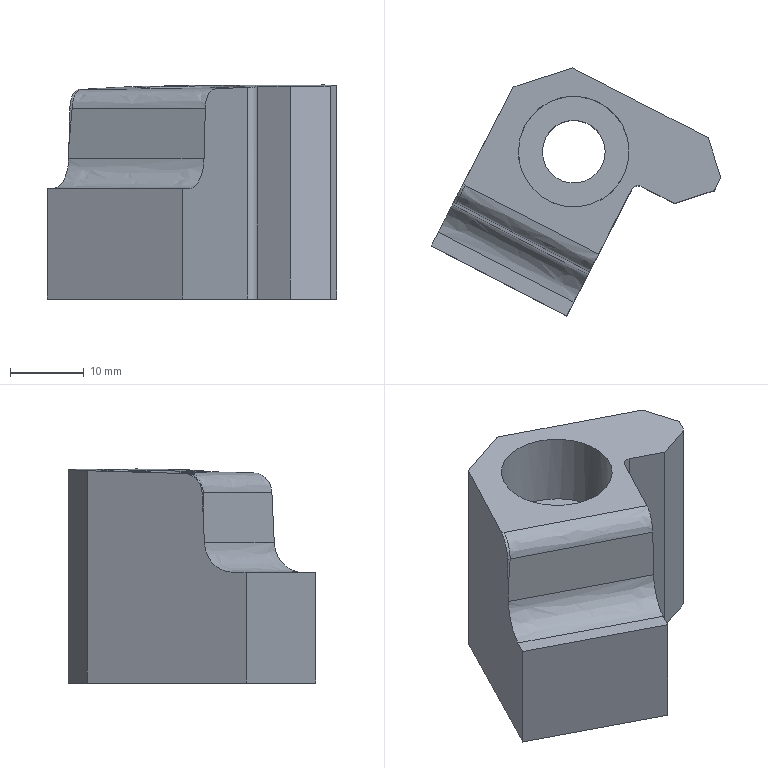Part | STEP file | gslz 2016.10.28-13_id1634_x_t | 1 solid | 21 faces | box 39.238 x 33.552 x 28.984 mm | volume 15189 mm3 | plane 12 | spline 5 | cylinder 4 | commonest cylinder face diameters 2 x1 8.5 x1 15 x1 21.5 x1